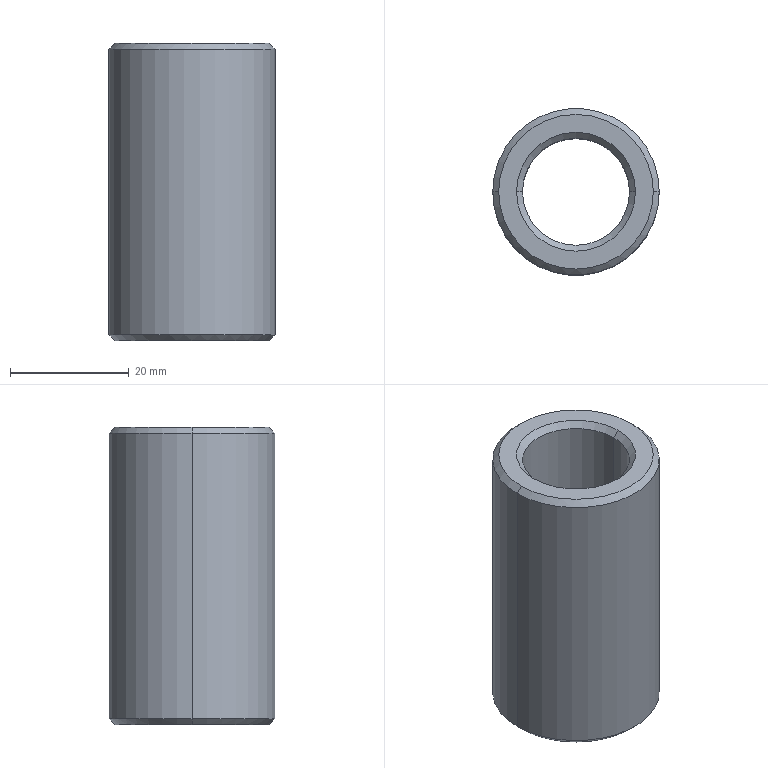Part | STEP file | VD-SYL0380DJ1006_1_1-15_2_VD-SY | 1 solid | 14 faces | box 28 x 28 x 50 mm | volume 17920 mm3 | cone 8 | cylinder 4 | plane 2 | commonest cylinder face diameters 18 x2 28 x2
STEP:
#1=CARTESIAN_POINT('',(9.,0.,-24.));
#2=VERTEX_POINT('',#1);
#3=CARTESIAN_POINT('',(-9.,0.,-24.));
#4=VERTEX_POINT('',#3);
#5=CARTESIAN_POINT('',(0.,0.,-24.));
#6=DIRECTION('',(0.,0.,1.));
#7=DIRECTION('',(1.,0.,0.));
#8=AXIS2_PLACEMENT_3D('',#5,#6,#7);
#9=CIRCLE('',#8,9.);
#10=EDGE_CURVE('',#2,#4,#9,.T.);
#11=ORIENTED_EDGE('',*,*,#10,.F.);
#12=CARTESIAN_POINT('',(9.,0.,24.));
#13=VERTEX_POINT('',#12);
#14=CARTESIAN_POINT('',(9.,0.,24.));
#15=DIRECTION('',(0.,0.,-1.));
#16=VECTOR('',#15,1000.);
#17=LINE('',#14,#16);
#18=EDGE_CURVE('',#13,#2,#17,.T.);
#19=ORIENTED_EDGE('',*,*,#18,.F.);
#20=CARTESIAN_POINT('',(-9.,0.,24.));
#21=VERTEX_POINT('',#20);
#22=CARTESIAN_POINT('',(0.,0.,24.));
#23=DIRECTION('',(0.,0.,-1.));
#24=DIRECTION('',(-1.,0.,0.));
#25=AXIS2_PLACEMENT_3D('',#22,#23,#24);
#26=CIRCLE('',#25,9.);
#27=EDGE_CURVE('',#21,#13,#26,.T.);
#28=ORIENTED_EDGE('',*,*,#27,.F.);
#29=CARTESIAN_POINT('',(-9.,0.,24.));
#30=DIRECTION('',(0.,0.,-1.));
#31=VECTOR('',#30,1000.);
#32=LINE('',#29,#31);
#33=EDGE_CURVE('',#21,#4,#32,.T.);
#34=ORIENTED_EDGE('',*,*,#33,.T.);
#35=EDGE_LOOP('',(#11,#19,#28,#34));
#36=FACE_OUTER_BOUND('',#35,.T.);
#37=CARTESIAN_POINT('',(0.,0.,-25.));
#38=DIRECTION('',(0.,0.,1.));
#39=DIRECTION('',(1.,0.,0.));
#40=AXIS2_PLACEMENT_3D('',#37,#38,#39);
#41=CYLINDRICAL_SURFACE('',#40,9.);
#42=ADVANCED_FACE('',(#36),#41,.F.);
#43=CARTESIAN_POINT('',(-13.,0.,25.));
#44=VERTEX_POINT('',#43);
#45=CARTESIAN_POINT('',(13.,0.,25.));
#46=VERTEX_POINT('',#45);
#47=CARTESIAN_POINT('',(0.,0.,25.));
#48=DIRECTION('',(0.,0.,1.));
#49=DIRECTION('',(-1.,0.,0.));
#50=AXIS2_PLACEMENT_3D('',#47,#48,#49);
#51=CIRCLE('',#50,13.);
#52=EDGE_CURVE('',#44,#46,#51,.T.);
#53=ORIENTED_EDGE('',*,*,#52,.F.);
#54=CARTESIAN_POINT('',(-14.,0.,24.));
#55=VERTEX_POINT('',#54);
#56=CARTESIAN_POINT('',(-14.,0.,24.));
#57=DIRECTION('',(0.7071,0.,0.7071));
#58=VECTOR('',#57,1000.);
#59=LINE('',#56,#58);
#60=EDGE_CURVE('',#55,#44,#59,.T.);
#61=ORIENTED_EDGE('',*,*,#60,.F.);
#62=CARTESIAN_POINT('',(14.,0.,24.));
#63=VERTEX_POINT('',#62);
#64=CARTESIAN_POINT('',(0.,0.,24.));
#65=DIRECTION('',(0.,0.,1.));
#66=DIRECTION('',(-1.,0.,0.));
#67=AXIS2_PLACEMENT_3D('',#64,#65,#66);
#68=CIRCLE('',#67,14.);
#69=EDGE_CURVE('',#55,#63,#68,.T.);
#70=ORIENTED_EDGE('',*,*,#69,.T.);
#71=CARTESIAN_POINT('',(14.,0.,24.));
#72=DIRECTION('',(-0.7071,0.,0.7071));
#73=VECTOR('',#72,1000.);
#74=LINE('',#71,#73);
#75=EDGE_CURVE('',#63,#46,#74,.T.);
#76=ORIENTED_EDGE('',*,*,#75,.T.);
#77=EDGE_LOOP('',(#53,#61,#70,#76));
#78=FACE_OUTER_BOUND('',#77,.T.);
#79=CARTESIAN_POINT('',(0.,0.,24.5));
#80=DIRECTION('',(0.,0.,-1.));
#81=DIRECTION('',(-1.,0.,0.));
#82=AXIS2_PLACEMENT_3D('',#79,#80,#81);
#83=CONICAL_SURFACE('',#82,13.5,0.7854);
#84=ADVANCED_FACE('',(#78),#83,.T.);
#85=CARTESIAN_POINT('',(-10.,0.,25.));
#86=VERTEX_POINT('',#85);
#87=CARTESIAN_POINT('',(10.,0.,25.));
#88=VERTEX_POINT('',#87);
#89=CARTESIAN_POINT('',(0.,0.,25.));
#90=DIRECTION('',(0.,0.,-1.));
#91=DIRECTION('',(-1.,0.,0.));
#92=AXIS2_PLACEMENT_3D('',#89,#90,#91);
#93=CIRCLE('',#92,10.);
#94=EDGE_CURVE('',#86,#88,#93,.T.);
#95=ORIENTED_EDGE('',*,*,#94,.T.);
#96=CARTESIAN_POINT('',(0.,0.,25.));
#97=DIRECTION('',(0.,0.,-1.));
#98=DIRECTION('',(1.,0.,0.));
#99=AXIS2_PLACEMENT_3D('',#96,#97,#98);
#100=CIRCLE('',#99,10.);
#101=EDGE_CURVE('',#88,#86,#100,.T.);
#102=ORIENTED_EDGE('',*,*,#101,.T.);
#103=EDGE_LOOP('',(#95,#102));
#104=FACE_BOUND('',#103,.T.);
#105=ORIENTED_EDGE('',*,*,#52,.T.);
#106=CARTESIAN_POINT('',(0.,0.,25.));
#107=DIRECTION('',(0.,0.,1.));
#108=DIRECTION('',(1.,0.,0.));
#109=AXIS2_PLACEMENT_3D('',#106,#107,#108);
#110=CIRCLE('',#109,13.);
#111=EDGE_CURVE('',#46,#44,#110,.T.);
#112=ORIENTED_EDGE('',*,*,#111,.T.);
#113=EDGE_LOOP('',(#105,#112));
#114=FACE_OUTER_BOUND('',#113,.T.);
#115=CARTESIAN_POINT('',(0.,0.,25.));
#116=DIRECTION('',(0.,0.,1.));
#117=DIRECTION('',(1.,0.,0.));
#118=AXIS2_PLACEMENT_3D('',#115,#116,#117);
#119=PLANE('',#118);
#120=ADVANCED_FACE('',(#104,#114),#119,.T.);
#121=ORIENTED_EDGE('',*,*,#75,.F.);
#122=CARTESIAN_POINT('',(0.,0.,24.));
#123=DIRECTION('',(0.,0.,1.));
#124=DIRECTION('',(1.,0.,0.));
#125=AXIS2_PLACEMENT_3D('',#122,#123,#124);
#126=CIRCLE('',#125,14.);
#127=EDGE_CURVE('',#63,#55,#126,.T.);
#128=ORIENTED_EDGE('',*,*,#127,.T.);
#129=ORIENTED_EDGE('',*,*,#60,.T.);
#130=ORIENTED_EDGE('',*,*,#111,.F.);
#131=EDGE_LOOP('',(#121,#128,#129,#130));
#132=FACE_OUTER_BOUND('',#131,.T.);
#133=CARTESIAN_POINT('',(0.,0.,24.5));
#134=DIRECTION('',(0.,0.,-1.));
#135=DIRECTION('',(-1.,0.,0.));
#136=AXIS2_PLACEMENT_3D('',#133,#134,#135);
#137=CONICAL_SURFACE('',#136,13.5,0.7854);
#138=ADVANCED_FACE('',(#132),#137,.T.);
#139=CARTESIAN_POINT('',(-14.,0.,-24.));
#140=VERTEX_POINT('',#139);
#141=CARTESIAN_POINT('',(-14.,0.,24.));
#142=DIRECTION('',(0.,0.,-1.));
#143=VECTOR('',#142,1000.);
#144=LINE('',#141,#143);
#145=EDGE_CURVE('',#55,#140,#144,.T.);
#146=ORIENTED_EDGE('',*,*,#145,.F.);
#147=ORIENTED_EDGE('',*,*,#127,.F.);
#148=CARTESIAN_POINT('',(14.,0.,-24.));
#149=VERTEX_POINT('',#148);
#150=CARTESIAN_POINT('',(14.,0.,24.));
#151=DIRECTION('',(0.,0.,-1.));
#152=VECTOR('',#151,1000.);
#153=LINE('',#150,#152);
#154=EDGE_CURVE('',#63,#149,#153,.T.);
#155=ORIENTED_EDGE('',*,*,#154,.T.);
#156=CARTESIAN_POINT('',(0.,0.,-24.));
#157=DIRECTION('',(0.,0.,-1.));
#158=DIRECTION('',(-1.,0.,0.));
#159=AXIS2_PLACEMENT_3D('',#156,#157,#158);
#160=CIRCLE('',#159,14.);
#161=EDGE_CURVE('',#140,#149,#160,.T.);
#162=ORIENTED_EDGE('',*,*,#161,.F.);
#163=EDGE_LOOP('',(#146,#147,#155,#162));
#164=FACE_OUTER_BOUND('',#163,.T.);
#165=CARTESIAN_POINT('',(0.,0.,-25.));
#166=DIRECTION('',(0.,0.,1.));
#167=DIRECTION('',(1.,0.,0.));
#168=AXIS2_PLACEMENT_3D('',#165,#166,#167);
#169=CYLINDRICAL_SURFACE('',#168,14.);
#170=ADVANCED_FACE('',(#164),#169,.T.);
#171=CARTESIAN_POINT('',(0.,0.,-24.));
#172=DIRECTION('',(0.,0.,-1.));
#173=DIRECTION('',(1.,0.,0.));
#174=AXIS2_PLACEMENT_3D('',#171,#172,#173);
#175=CIRCLE('',#174,14.);
#176=EDGE_CURVE('',#149,#140,#175,.T.);
#177=ORIENTED_EDGE('',*,*,#176,.F.);
#178=ORIENTED_EDGE('',*,*,#154,.F.);
#179=ORIENTED_EDGE('',*,*,#69,.F.);
#180=ORIENTED_EDGE('',*,*,#145,.T.);
#181=EDGE_LOOP('',(#177,#178,#179,#180));
#182=FACE_OUTER_BOUND('',#181,.T.);
#183=CARTESIAN_POINT('',(0.,0.,-25.));
#184=DIRECTION('',(0.,0.,1.));
#185=DIRECTION('',(1.,0.,0.));
#186=AXIS2_PLACEMENT_3D('',#183,#184,#185);
#187=CYLINDRICAL_SURFACE('',#186,14.);
#188=ADVANCED_FACE('',(#182),#187,.T.);
#189=CARTESIAN_POINT('',(13.,0.,-25.));
#190=VERTEX_POINT('',#189);
#191=CARTESIAN_POINT('',(-13.,0.,-25.));
#192=VERTEX_POINT('',#191);
#193=CARTESIAN_POINT('',(0.,0.,-25.));
#194=DIRECTION('',(0.,0.,-1.));
#195=DIRECTION('',(1.,0.,0.));
#196=AXIS2_PLACEMENT_3D('',#193,#194,#195);
#197=CIRCLE('',#196,13.);
#198=EDGE_CURVE('',#190,#192,#197,.T.);
#199=ORIENTED_EDGE('',*,*,#198,.F.);
#200=CARTESIAN_POINT('',(14.,0.,-24.));
#201=DIRECTION('',(-0.7071,0.,-0.7071));
#202=VECTOR('',#201,1000.);
#203=LINE('',#200,#202);
#204=EDGE_CURVE('',#149,#190,#203,.T.);
#205=ORIENTED_EDGE('',*,*,#204,.F.);
#206=ORIENTED_EDGE('',*,*,#176,.T.);
#207=CARTESIAN_POINT('',(-14.,0.,-24.));
#208=DIRECTION('',(0.7071,0.,-0.7071));
#209=VECTOR('',#208,1000.);
#210=LINE('',#207,#209);
#211=EDGE_CURVE('',#140,#192,#210,.T.);
#212=ORIENTED_EDGE('',*,*,#211,.T.);
#213=EDGE_LOOP('',(#199,#205,#206,#212));
#214=FACE_OUTER_BOUND('',#213,.T.);
#215=CARTESIAN_POINT('',(0.,0.,-24.5));
#216=DIRECTION('',(0.,0.,1.));
#217=DIRECTION('',(1.,0.,0.));
#218=AXIS2_PLACEMENT_3D('',#215,#216,#217);
#219=CONICAL_SURFACE('',#218,13.5,0.7854);
#220=ADVANCED_FACE('',(#214),#219,.T.);
#221=ORIENTED_EDGE('',*,*,#211,.F.);
#222=ORIENTED_EDGE('',*,*,#161,.T.);
#223=ORIENTED_EDGE('',*,*,#204,.T.);
#224=CARTESIAN_POINT('',(0.,0.,-25.));
#225=DIRECTION('',(0.,0.,-1.));
#226=DIRECTION('',(-1.,0.,0.));
#227=AXIS2_PLACEMENT_3D('',#224,#225,#226);
#228=CIRCLE('',#227,13.);
#229=EDGE_CURVE('',#192,#190,#228,.T.);
#230=ORIENTED_EDGE('',*,*,#229,.F.);
#231=EDGE_LOOP('',(#221,#222,#223,#230));
#232=FACE_OUTER_BOUND('',#231,.T.);
#233=CARTESIAN_POINT('',(0.,0.,-24.5));
#234=DIRECTION('',(0.,0.,1.));
#235=DIRECTION('',(1.,0.,0.));
#236=AXIS2_PLACEMENT_3D('',#233,#234,#235);
#237=CONICAL_SURFACE('',#236,13.5,0.7854);
#238=ADVANCED_FACE('',(#232),#237,.T.);
#239=CARTESIAN_POINT('',(-10.,0.,-25.));
#240=VERTEX_POINT('',#239);
#241=CARTESIAN_POINT('',(10.,0.,-25.));
#242=VERTEX_POINT('',#241);
#243=CARTESIAN_POINT('',(0.,0.,-25.));
#244=DIRECTION('',(0.,0.,1.));
#245=DIRECTION('',(-1.,0.,0.));
#246=AXIS2_PLACEMENT_3D('',#243,#244,#245);
#247=CIRCLE('',#246,10.);
#248=EDGE_CURVE('',#240,#242,#247,.T.);
#249=ORIENTED_EDGE('',*,*,#248,.T.);
#250=CARTESIAN_POINT('',(0.,0.,-25.));
#251=DIRECTION('',(0.,0.,1.));
#252=DIRECTION('',(1.,0.,0.));
#253=AXIS2_PLACEMENT_3D('',#250,#251,#252);
#254=CIRCLE('',#253,10.);
#255=EDGE_CURVE('',#242,#240,#254,.T.);
#256=ORIENTED_EDGE('',*,*,#255,.T.);
#257=EDGE_LOOP('',(#249,#256));
#258=FACE_BOUND('',#257,.T.);
#259=ORIENTED_EDGE('',*,*,#198,.T.);
#260=ORIENTED_EDGE('',*,*,#229,.T.);
#261=EDGE_LOOP('',(#259,#260));
#262=FACE_OUTER_BOUND('',#261,.T.);
#263=CARTESIAN_POINT('',(0.,0.,-25.));
#264=DIRECTION('',(0.,0.,1.));
#265=DIRECTION('',(1.,0.,0.));
#266=AXIS2_PLACEMENT_3D('',#263,#264,#265);
#267=PLANE('',#266);
#268=ADVANCED_FACE('',(#258,#262),#267,.F.);
#269=ORIENTED_EDGE('',*,*,#10,.T.);
#270=CARTESIAN_POINT('',(-10.,0.,-25.));
#271=DIRECTION('',(0.7071,0.,0.7071));
#272=VECTOR('',#271,1000.);
#273=LINE('',#270,#272);
#274=EDGE_CURVE('',#240,#4,#273,.T.);
#275=ORIENTED_EDGE('',*,*,#274,.F.);
#276=ORIENTED_EDGE('',*,*,#255,.F.);
#277=CARTESIAN_POINT('',(10.,0.,-25.));
#278=DIRECTION('',(-0.7071,0.,0.7071));
#279=VECTOR('',#278,1000.);
#280=LINE('',#277,#279);
#281=EDGE_CURVE('',#242,#2,#280,.T.);
#282=ORIENTED_EDGE('',*,*,#281,.T.);
#283=EDGE_LOOP('',(#269,#275,#276,#282));
#284=FACE_OUTER_BOUND('',#283,.T.);
#285=CARTESIAN_POINT('',(0.,0.,-24.5));
#286=DIRECTION('',(0.,0.,-1.));
#287=DIRECTION('',(-1.,0.,0.));
#288=AXIS2_PLACEMENT_3D('',#285,#286,#287);
#289=CONICAL_SURFACE('',#288,9.5,0.7854);
#290=ADVANCED_FACE('',(#284),#289,.F.);
#291=ORIENTED_EDGE('',*,*,#281,.F.);
#292=ORIENTED_EDGE('',*,*,#248,.F.);
#293=ORIENTED_EDGE('',*,*,#274,.T.);
#294=CARTESIAN_POINT('',(0.,0.,-24.));
#295=DIRECTION('',(0.,0.,1.));
#296=DIRECTION('',(-1.,0.,0.));
#297=AXIS2_PLACEMENT_3D('',#294,#295,#296);
#298=CIRCLE('',#297,9.);
#299=EDGE_CURVE('',#4,#2,#298,.T.);
#300=ORIENTED_EDGE('',*,*,#299,.T.);
#301=EDGE_LOOP('',(#291,#292,#293,#300));
#302=FACE_OUTER_BOUND('',#301,.T.);
#303=CARTESIAN_POINT('',(0.,0.,-24.5));
#304=DIRECTION('',(0.,0.,-1.));
#305=DIRECTION('',(-1.,0.,0.));
#306=AXIS2_PLACEMENT_3D('',#303,#304,#305);
#307=CONICAL_SURFACE('',#306,9.5,0.7854);
#308=ADVANCED_FACE('',(#302),#307,.F.);
#309=ORIENTED_EDGE('',*,*,#33,.F.);
#310=CARTESIAN_POINT('',(0.,0.,24.));
#311=DIRECTION('',(0.,0.,-1.));
#312=DIRECTION('',(1.,0.,0.));
#313=AXIS2_PLACEMENT_3D('',#310,#311,#312);
#314=CIRCLE('',#313,9.);
#315=EDGE_CURVE('',#13,#21,#314,.T.);
#316=ORIENTED_EDGE('',*,*,#315,.F.);
#317=ORIENTED_EDGE('',*,*,#18,.T.);
#318=ORIENTED_EDGE('',*,*,#299,.F.);
#319=EDGE_LOOP('',(#309,#316,#317,#318));
#320=FACE_OUTER_BOUND('',#319,.T.);
#321=CARTESIAN_POINT('',(0.,0.,-25.));
#322=DIRECTION('',(0.,0.,1.));
#323=DIRECTION('',(1.,0.,0.));
#324=AXIS2_PLACEMENT_3D('',#321,#322,#323);
#325=CYLINDRICAL_SURFACE('',#324,9.);
#326=ADVANCED_FACE('',(#320),#325,.F.);
#327=CARTESIAN_POINT('',(-10.,0.,25.));
#328=DIRECTION('',(0.7071,0.,-0.7071));
#329=VECTOR('',#328,1000.);
#330=LINE('',#327,#329);
#331=EDGE_CURVE('',#86,#21,#330,.T.);
#332=ORIENTED_EDGE('',*,*,#331,.F.);
#333=ORIENTED_EDGE('',*,*,#101,.F.);
#334=CARTESIAN_POINT('',(10.,0.,25.));
#335=DIRECTION('',(-0.7071,0.,-0.7071));
#336=VECTOR('',#335,1000.);
#337=LINE('',#334,#336);
#338=EDGE_CURVE('',#88,#13,#337,.T.);
#339=ORIENTED_EDGE('',*,*,#338,.T.);
#340=ORIENTED_EDGE('',*,*,#315,.T.);
#341=EDGE_LOOP('',(#332,#333,#339,#340));
#342=FACE_OUTER_BOUND('',#341,.T.);
#343=CARTESIAN_POINT('',(0.,0.,24.5));
#344=DIRECTION('',(0.,0.,1.));
#345=DIRECTION('',(1.,0.,0.));
#346=AXIS2_PLACEMENT_3D('',#343,#344,#345);
#347=CONICAL_SURFACE('',#346,9.5,0.7854);
#348=ADVANCED_FACE('',(#342),#347,.F.);
#349=ORIENTED_EDGE('',*,*,#27,.T.);
#350=ORIENTED_EDGE('',*,*,#338,.F.);
#351=ORIENTED_EDGE('',*,*,#94,.F.);
#352=ORIENTED_EDGE('',*,*,#331,.T.);
#353=EDGE_LOOP('',(#349,#350,#351,#352));
#354=FACE_OUTER_BOUND('',#353,.T.);
#355=CARTESIAN_POINT('',(0.,0.,24.5));
#356=DIRECTION('',(0.,0.,1.));
#357=DIRECTION('',(1.,0.,0.));
#358=AXIS2_PLACEMENT_3D('',#355,#356,#357);
#359=CONICAL_SURFACE('',#358,9.5,0.7854);
#360=ADVANCED_FACE('',(#354),#359,.F.);
#361=CLOSED_SHELL('',(#42,#84,#120,#138,#170,#188,#220,#238,#268,#290,#308,#326,#348,#360));
#362=MANIFOLD_SOLID_BREP('',#361);
#363=CARTESIAN_POINT('',(0.,0.,0.));
#364=DIRECTION('',(0.,0.,1.));
#365=DIRECTION('',(1.,0.,0.));
#366=AXIS2_PLACEMENT_3D('',#363,#364,#365);
#367=(LENGTH_UNIT()NAMED_UNIT(*)SI_UNIT(.MILLI.,.METRE.));
#368=UNCERTAINTY_MEASURE_WITH_UNIT(LENGTH_MEASURE(0.00001),#367,'','');
#369=(NAMED_UNIT(*)PLANE_ANGLE_UNIT()SI_UNIT($,.RADIAN.));
#370=(NAMED_UNIT(*)SI_UNIT($,.STERADIAN.)SOLID_ANGLE_UNIT());
#371=(GEOMETRIC_REPRESENTATION_CONTEXT(3)GLOBAL_UNCERTAINTY_ASSIGNED_CONTEXT((#368))GLOBAL_UNIT_ASSIGNED_CONTEXT((#367,#369,#370))REPRESENTATION_CONTEXT('',''));
#372=ADVANCED_BREP_SHAPE_REPRESENTATION('',(#362,#366),#371);